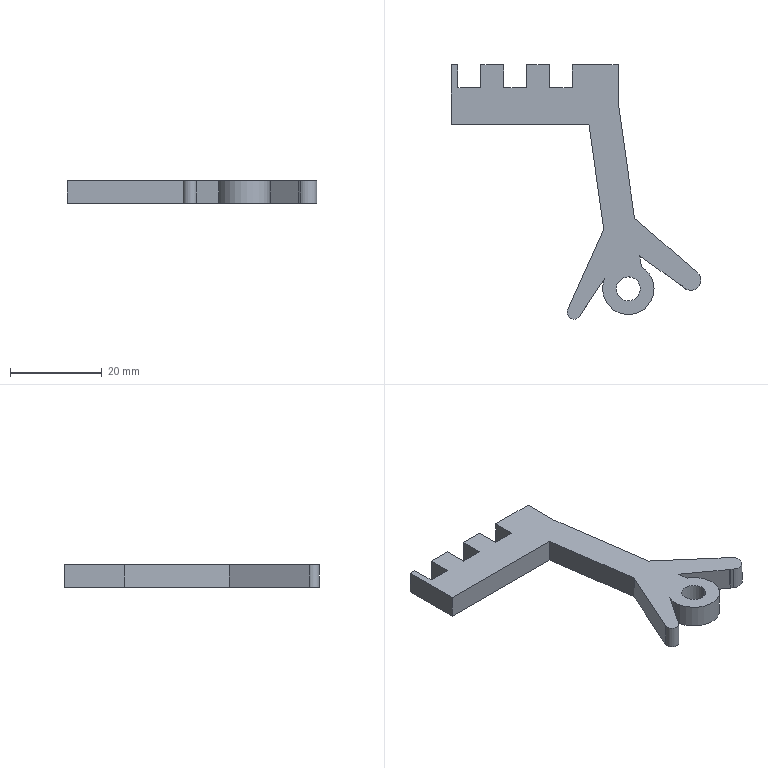Part | SolidWorks | features ICE 28, Join 2 | 1 solid | 34 faces | box 54.608 x 55.606 x 5 mm | volume 4241 mm3 | plane 27 | cylinder 7 | commonest cylinder face diameters 11.246 x3 5.25 x2 3 x1 4.42 x1
STEP:
#1=CARTESIAN_POINT('',(28.531,-18.492,-5.));
#2=VERTEX_POINT('',#1);
#3=CARTESIAN_POINT('',(28.044,-20.781,-5.));
#4=VERTEX_POINT('',#3);
#5=CARTESIAN_POINT('',(33.667,-20.781,-5.));
#6=DIRECTION('',(0.,0.,1.));
#7=DIRECTION('',(-1.,0.,0.));
#8=AXIS2_PLACEMENT_3D('',#5,#6,#7);
#9=CIRCLE('',#8,5.623);
#10=EDGE_CURVE('',#2,#4,#9,.T.);
#11=ORIENTED_EDGE('',*,*,#10,.T.);
#12=CARTESIAN_POINT('',(28.044,-20.781,0.));
#13=VERTEX_POINT('',#12);
#14=CARTESIAN_POINT('',(28.044,-20.781,-20.904));
#15=DIRECTION('',(0.,0.,1.));
#16=VECTOR('',#15,1000.);
#17=LINE('',#14,#16);
#18=EDGE_CURVE('',#4,#13,#17,.T.);
#19=ORIENTED_EDGE('',*,*,#18,.T.);
#20=CARTESIAN_POINT('',(28.531,-18.492,0.));
#21=VERTEX_POINT('',#20);
#22=CARTESIAN_POINT('',(33.667,-20.781,0.));
#23=DIRECTION('',(0.,0.,1.));
#24=DIRECTION('',(1.,0.,0.));
#25=AXIS2_PLACEMENT_3D('',#22,#23,#24);
#26=CIRCLE('',#25,5.623);
#27=EDGE_CURVE('',#21,#13,#26,.T.);
#28=ORIENTED_EDGE('',*,*,#27,.F.);
#29=CARTESIAN_POINT('',(28.531,-18.492,-20.904));
#30=DIRECTION('',(0.,0.,-1.));
#31=VECTOR('',#30,1000.);
#32=LINE('',#29,#31);
#33=EDGE_CURVE('',#21,#2,#32,.T.);
#34=ORIENTED_EDGE('',*,*,#33,.T.);
#35=EDGE_LOOP('',(#11,#19,#28,#34));
#36=FACE_OUTER_BOUND('',#35,.T.);
#37=CARTESIAN_POINT('',(33.667,-20.781,-20.904));
#38=DIRECTION('',(0.,0.,1.));
#39=DIRECTION('',(1.,0.,0.));
#40=AXIS2_PLACEMENT_3D('',#37,#38,#39);
#41=CYLINDRICAL_SURFACE('',#40,5.623);
#42=ADVANCED_FACE('',(#36),#41,.T.);
#43=ORIENTED_EDGE('',*,*,#18,.F.);
#44=CARTESIAN_POINT('',(39.29,-20.781,-5.));
#45=VERTEX_POINT('',#44);
#46=CARTESIAN_POINT('',(33.667,-20.781,-5.));
#47=DIRECTION('',(0.,0.,1.));
#48=DIRECTION('',(-1.,0.,0.));
#49=AXIS2_PLACEMENT_3D('',#46,#47,#48);
#50=CIRCLE('',#49,5.623);
#51=EDGE_CURVE('',#4,#45,#50,.T.);
#52=ORIENTED_EDGE('',*,*,#51,.T.);
#53=CARTESIAN_POINT('',(39.29,-20.781,0.));
#54=VERTEX_POINT('',#53);
#55=CARTESIAN_POINT('',(39.29,-20.781,-20.904));
#56=DIRECTION('',(0.,0.,1.));
#57=VECTOR('',#56,1000.);
#58=LINE('',#55,#57);
#59=EDGE_CURVE('',#45,#54,#58,.T.);
#60=ORIENTED_EDGE('',*,*,#59,.T.);
#61=CARTESIAN_POINT('',(33.667,-20.781,0.));
#62=DIRECTION('',(0.,0.,1.));
#63=DIRECTION('',(1.,0.,0.));
#64=AXIS2_PLACEMENT_3D('',#61,#62,#63);
#65=CIRCLE('',#64,5.623);
#66=EDGE_CURVE('',#13,#54,#65,.T.);
#67=ORIENTED_EDGE('',*,*,#66,.F.);
#68=EDGE_LOOP('',(#43,#52,#60,#67));
#69=FACE_OUTER_BOUND('',#68,.T.);
#70=CARTESIAN_POINT('',(33.667,-20.781,-20.904));
#71=DIRECTION('',(0.,0.,1.));
#72=DIRECTION('',(1.,0.,0.));
#73=AXIS2_PLACEMENT_3D('',#70,#71,#72);
#74=CYLINDRICAL_SURFACE('',#73,5.623);
#75=ADVANCED_FACE('',(#69),#74,.T.);
#76=CARTESIAN_POINT('',(36.277,-21.054,-5.));
#77=VERTEX_POINT('',#76);
#78=CARTESIAN_POINT('',(31.056,-20.508,-5.));
#79=VERTEX_POINT('',#78);
#80=CARTESIAN_POINT('',(33.667,-20.781,-5.));
#81=DIRECTION('',(0.,0.,-1.));
#82=DIRECTION('',(-0.9946,0.1041,0.));
#83=AXIS2_PLACEMENT_3D('',#80,#81,#82);
#84=CIRCLE('',#83,2.625);
#85=EDGE_CURVE('',#77,#79,#84,.T.);
#86=ORIENTED_EDGE('',*,*,#85,.T.);
#87=CARTESIAN_POINT('',(31.056,-20.508,0.));
#88=VERTEX_POINT('',#87);
#89=CARTESIAN_POINT('',(31.056,-20.508,-10.));
#90=DIRECTION('',(0.,0.,1.));
#91=VECTOR('',#90,1000.);
#92=LINE('',#89,#91);
#93=EDGE_CURVE('',#79,#88,#92,.T.);
#94=ORIENTED_EDGE('',*,*,#93,.T.);
#95=CARTESIAN_POINT('',(36.277,-21.054,0.));
#96=VERTEX_POINT('',#95);
#97=CARTESIAN_POINT('',(33.667,-20.781,0.));
#98=DIRECTION('',(0.,0.,1.));
#99=DIRECTION('',(0.9946,-0.1041,0.));
#100=AXIS2_PLACEMENT_3D('',#97,#98,#99);
#101=CIRCLE('',#100,2.625);
#102=EDGE_CURVE('',#88,#96,#101,.T.);
#103=ORIENTED_EDGE('',*,*,#102,.T.);
#104=CARTESIAN_POINT('',(36.277,-21.054,-10.));
#105=DIRECTION('',(0.,0.,1.));
#106=VECTOR('',#105,1000.);
#107=LINE('',#104,#106);
#108=EDGE_CURVE('',#77,#96,#107,.T.);
#109=ORIENTED_EDGE('',*,*,#108,.F.);
#110=EDGE_LOOP('',(#86,#94,#103,#109));
#111=FACE_OUTER_BOUND('',#110,.T.);
#112=CARTESIAN_POINT('',(33.667,-20.781,-10.));
#113=DIRECTION('',(0.,0.,1.));
#114=DIRECTION('',(0.9946,-0.1041,0.));
#115=AXIS2_PLACEMENT_3D('',#112,#113,#114);
#116=CYLINDRICAL_SURFACE('',#115,2.625);
#117=ADVANCED_FACE('',(#111),#116,.F.);
#118=CARTESIAN_POINT('',(-5.057,28.192,0.));
#119=VERTEX_POINT('',#118);
#120=CARTESIAN_POINT('',(-5.057,28.192,-5.));
#121=VERTEX_POINT('',#120);
#122=CARTESIAN_POINT('',(-5.057,28.192,5.));
#123=DIRECTION('',(0.,0.,-1.));
#124=VECTOR('',#123,1000.);
#125=LINE('',#122,#124);
#126=EDGE_CURVE('',#119,#121,#125,.T.);
#127=ORIENTED_EDGE('',*,*,#126,.F.);
#128=CARTESIAN_POINT('',(-3.557,28.192,0.));
#129=VERTEX_POINT('',#128);
#130=CARTESIAN_POINT('',(-16.089,28.192,0.));
#131=DIRECTION('',(1.,0.,0.));
#132=VECTOR('',#131,1000.);
#133=LINE('',#130,#132);
#134=EDGE_CURVE('',#119,#129,#133,.T.);
#135=ORIENTED_EDGE('',*,*,#134,.T.);
#136=CARTESIAN_POINT('',(-3.557,28.192,-5.));
#137=VERTEX_POINT('',#136);
#138=CARTESIAN_POINT('',(-3.557,28.192,0.001));
#139=DIRECTION('',(0.,0.,-1.));
#140=VECTOR('',#139,1000.);
#141=LINE('',#138,#140);
#142=EDGE_CURVE('',#129,#137,#141,.T.);
#143=ORIENTED_EDGE('',*,*,#142,.T.);
#144=CARTESIAN_POINT('',(-16.089,28.192,-5.));
#145=DIRECTION('',(1.,0.,0.));
#146=VECTOR('',#145,1000.);
#147=LINE('',#144,#146);
#148=EDGE_CURVE('',#121,#137,#147,.T.);
#149=ORIENTED_EDGE('',*,*,#148,.F.);
#150=EDGE_LOOP('',(#127,#135,#143,#149));
#151=FACE_OUTER_BOUND('',#150,.T.);
#152=CARTESIAN_POINT('',(-16.089,28.192,-5.));
#153=DIRECTION('',(0.,-1.,0.));
#154=DIRECTION('',(0.,0.,-1.));
#155=AXIS2_PLACEMENT_3D('',#152,#153,#154);
#156=PLANE('',#155);
#157=ADVANCED_FACE('',(#151),#156,.F.);
#158=CARTESIAN_POINT('',(-5.057,15.192,0.));
#159=VERTEX_POINT('',#158);
#160=CARTESIAN_POINT('',(-5.057,15.192,-5.));
#161=VERTEX_POINT('',#160);
#162=CARTESIAN_POINT('',(-5.057,15.192,5.));
#163=DIRECTION('',(0.,0.,-1.));
#164=VECTOR('',#163,1000.);
#165=LINE('',#162,#164);
#166=EDGE_CURVE('',#159,#161,#165,.T.);
#167=ORIENTED_EDGE('',*,*,#166,.T.);
#168=CARTESIAN_POINT('',(25.077,15.192,-5.));
#169=VERTEX_POINT('',#168);
#170=CARTESIAN_POINT('',(-16.089,15.192,-5.));
#171=DIRECTION('',(1.,0.,0.));
#172=VECTOR('',#171,1000.);
#173=LINE('',#170,#172);
#174=EDGE_CURVE('',#161,#169,#173,.T.);
#175=ORIENTED_EDGE('',*,*,#174,.T.);
#176=CARTESIAN_POINT('',(25.077,15.192,0.));
#177=VERTEX_POINT('',#176);
#178=CARTESIAN_POINT('',(25.077,15.192,0.));
#179=DIRECTION('',(0.,0.,-1.));
#180=VECTOR('',#179,1000.);
#181=LINE('',#178,#180);
#182=EDGE_CURVE('',#177,#169,#181,.T.);
#183=ORIENTED_EDGE('',*,*,#182,.F.);
#184=CARTESIAN_POINT('',(-16.089,15.192,0.));
#185=DIRECTION('',(1.,0.,0.));
#186=VECTOR('',#185,1000.);
#187=LINE('',#184,#186);
#188=EDGE_CURVE('',#159,#177,#187,.T.);
#189=ORIENTED_EDGE('',*,*,#188,.F.);
#190=EDGE_LOOP('',(#167,#175,#183,#189));
#191=FACE_OUTER_BOUND('',#190,.T.);
#192=CARTESIAN_POINT('',(-16.089,15.192,-5.));
#193=DIRECTION('',(0.,1.,0.));
#194=DIRECTION('',(0.,0.,1.));
#195=AXIS2_PLACEMENT_3D('',#192,#193,#194);
#196=PLANE('',#195);
#197=ADVANCED_FACE('',(#191),#196,.F.);
#198=CARTESIAN_POINT('',(46.044,-20.68,-5.));
#199=VERTEX_POINT('',#198);
#200=CARTESIAN_POINT('',(48.785,-17.218,-5.));
#201=VERTEX_POINT('',#200);
#202=CARTESIAN_POINT('',(47.341,-18.89,-5.));
#203=DIRECTION('',(0.,0.,1.));
#204=DIRECTION('',(-1.,0.,0.));
#205=AXIS2_PLACEMENT_3D('',#202,#203,#204);
#206=CIRCLE('',#205,2.21);
#207=EDGE_CURVE('',#199,#201,#206,.T.);
#208=ORIENTED_EDGE('',*,*,#207,.F.);
#209=CARTESIAN_POINT('',(45.413,-20.127,-5.));
#210=VERTEX_POINT('',#209);
#211=CARTESIAN_POINT('',(45.413,-20.127,-5.));
#212=DIRECTION('',(0.7522,-0.6589,0.));
#213=VECTOR('',#212,1000.);
#214=LINE('',#211,#213);
#215=EDGE_CURVE('',#210,#199,#214,.T.);
#216=ORIENTED_EDGE('',*,*,#215,.F.);
#217=CARTESIAN_POINT('',(45.451,-20.251,-5.));
#218=VERTEX_POINT('',#217);
#219=CARTESIAN_POINT('',(46.236,-22.795,-5.));
#220=DIRECTION('',(-0.2947,0.9556,0.));
#221=VECTOR('',#220,1000.);
#222=LINE('',#219,#221);
#223=EDGE_CURVE('',#218,#210,#222,.T.);
#224=ORIENTED_EDGE('',*,*,#223,.F.);
#225=CARTESIAN_POINT('',(36.183,-13.539,-5.));
#226=VERTEX_POINT('',#225);
#227=CARTESIAN_POINT('',(3.892,9.847,-5.));
#228=DIRECTION('',(-0.8099,0.5865,0.));
#229=VECTOR('',#228,1000.);
#230=LINE('',#227,#229);
#231=EDGE_CURVE('',#218,#226,#230,.T.);
#232=ORIENTED_EDGE('',*,*,#231,.T.);
#233=CARTESIAN_POINT('',(36.52,-15.936,-5.));
#234=VERTEX_POINT('',#233);
#235=CARTESIAN_POINT('',(37.552,-23.275,-5.));
#236=DIRECTION('',(-0.1392,0.9903,0.));
#237=VECTOR('',#236,1000.);
#238=LINE('',#235,#237);
#239=EDGE_CURVE('',#234,#226,#238,.T.);
#240=ORIENTED_EDGE('',*,*,#239,.F.);
#241=CARTESIAN_POINT('',(33.667,-20.781,-5.));
#242=DIRECTION('',(0.,0.,1.));
#243=DIRECTION('',(-1.,0.,0.));
#244=AXIS2_PLACEMENT_3D('',#241,#242,#243);
#245=CIRCLE('',#244,5.623);
#246=EDGE_CURVE('',#45,#234,#245,.T.);
#247=ORIENTED_EDGE('',*,*,#246,.F.);
#248=ORIENTED_EDGE('',*,*,#51,.F.);
#249=ORIENTED_EDGE('',*,*,#10,.F.);
#250=CARTESIAN_POINT('',(23.157,-26.529,-5.));
#251=VERTEX_POINT('',#250);
#252=CARTESIAN_POINT('',(23.157,-26.529,-5.));
#253=DIRECTION('',(0.5558,0.8313,0.));
#254=VECTOR('',#253,1000.);
#255=LINE('',#252,#254);
#256=EDGE_CURVE('',#251,#2,#255,.T.);
#257=ORIENTED_EDGE('',*,*,#256,.F.);
#258=CARTESIAN_POINT('',(20.421,-25.3,-5.));
#259=VERTEX_POINT('',#258);
#260=CARTESIAN_POINT('',(21.789,-25.914,-5.));
#261=DIRECTION('',(0.,0.,1.));
#262=DIRECTION('',(0.9903,0.1392,0.));
#263=AXIS2_PLACEMENT_3D('',#260,#261,#262);
#264=CIRCLE('',#263,1.5);
#265=EDGE_CURVE('',#259,#251,#264,.T.);
#266=ORIENTED_EDGE('',*,*,#265,.F.);
#267=CARTESIAN_POINT('',(28.302,-7.759,-5.));
#268=VERTEX_POINT('',#267);
#269=CARTESIAN_POINT('',(28.302,-7.759,-5.));
#270=DIRECTION('',(-0.4099,-0.9121,0.));
#271=VECTOR('',#270,1000.);
#272=LINE('',#269,#271);
#273=EDGE_CURVE('',#268,#259,#272,.T.);
#274=ORIENTED_EDGE('',*,*,#273,.F.);
#275=CARTESIAN_POINT('',(30.62,-24.249,-5.));
#276=DIRECTION('',(0.1392,-0.9903,0.));
#277=VECTOR('',#276,1000.);
#278=LINE('',#275,#277);
#279=EDGE_CURVE('',#169,#268,#278,.T.);
#280=ORIENTED_EDGE('',*,*,#279,.F.);
#281=ORIENTED_EDGE('',*,*,#174,.F.);
#282=CARTESIAN_POINT('',(-5.057,0.,-5.));
#283=DIRECTION('',(0.,1.,0.));
#284=VECTOR('',#283,1000.);
#285=LINE('',#282,#284);
#286=EDGE_CURVE('',#161,#121,#285,.T.);
#287=ORIENTED_EDGE('',*,*,#286,.T.);
#288=ORIENTED_EDGE('',*,*,#148,.T.);
#289=CARTESIAN_POINT('',(-3.557,23.192,-5.));
#290=VERTEX_POINT('',#289);
#291=CARTESIAN_POINT('',(-3.557,28.192,-5.));
#292=DIRECTION('',(0.,1.,0.));
#293=VECTOR('',#292,1000.);
#294=LINE('',#291,#293);
#295=EDGE_CURVE('',#290,#137,#294,.T.);
#296=ORIENTED_EDGE('',*,*,#295,.F.);
#297=CARTESIAN_POINT('',(1.443,23.192,-5.));
#298=VERTEX_POINT('',#297);
#299=CARTESIAN_POINT('',(1.443,23.192,-5.));
#300=DIRECTION('',(-1.,0.,0.));
#301=VECTOR('',#300,1000.);
#302=LINE('',#299,#301);
#303=EDGE_CURVE('',#298,#290,#302,.T.);
#304=ORIENTED_EDGE('',*,*,#303,.F.);
#305=CARTESIAN_POINT('',(1.443,28.192,-5.));
#306=VERTEX_POINT('',#305);
#307=CARTESIAN_POINT('',(1.443,28.192,-5.));
#308=DIRECTION('',(0.,-1.,0.));
#309=VECTOR('',#308,1000.);
#310=LINE('',#307,#309);
#311=EDGE_CURVE('',#306,#298,#310,.T.);
#312=ORIENTED_EDGE('',*,*,#311,.F.);
#313=CARTESIAN_POINT('',(6.443,28.192,-5.));
#314=VERTEX_POINT('',#313);
#315=CARTESIAN_POINT('',(-16.089,28.192,-5.));
#316=DIRECTION('',(1.,0.,0.));
#317=VECTOR('',#316,1000.);
#318=LINE('',#315,#317);
#319=EDGE_CURVE('',#306,#314,#318,.T.);
#320=ORIENTED_EDGE('',*,*,#319,.T.);
#321=CARTESIAN_POINT('',(6.443,23.192,-5.));
#322=VERTEX_POINT('',#321);
#323=CARTESIAN_POINT('',(6.443,28.192,-5.));
#324=DIRECTION('',(0.,1.,0.));
#325=VECTOR('',#324,1000.);
#326=LINE('',#323,#325);
#327=EDGE_CURVE('',#322,#314,#326,.T.);
#328=ORIENTED_EDGE('',*,*,#327,.F.);
#329=CARTESIAN_POINT('',(11.443,23.192,-5.));
#330=VERTEX_POINT('',#329);
#331=CARTESIAN_POINT('',(6.443,23.192,-5.));
#332=DIRECTION('',(-1.,0.,0.));
#333=VECTOR('',#332,1000.);
#334=LINE('',#331,#333);
#335=EDGE_CURVE('',#330,#322,#334,.T.);
#336=ORIENTED_EDGE('',*,*,#335,.F.);
#337=CARTESIAN_POINT('',(11.443,28.192,-5.));
#338=VERTEX_POINT('',#337);
#339=CARTESIAN_POINT('',(11.443,28.192,-5.));
#340=DIRECTION('',(0.,-1.,0.));
#341=VECTOR('',#340,1000.);
#342=LINE('',#339,#341);
#343=EDGE_CURVE('',#338,#330,#342,.T.);
#344=ORIENTED_EDGE('',*,*,#343,.F.);
#345=CARTESIAN_POINT('',(16.443,28.192,-5.));
#346=VERTEX_POINT('',#345);
#347=CARTESIAN_POINT('',(-16.089,28.192,-5.));
#348=DIRECTION('',(1.,0.,0.));
#349=VECTOR('',#348,1000.);
#350=LINE('',#347,#349);
#351=EDGE_CURVE('',#338,#346,#350,.T.);
#352=ORIENTED_EDGE('',*,*,#351,.T.);
#353=CARTESIAN_POINT('',(16.443,23.192,-5.));
#354=VERTEX_POINT('',#353);
#355=CARTESIAN_POINT('',(16.443,28.192,-5.));
#356=DIRECTION('',(0.,1.,0.));
#357=VECTOR('',#356,1000.);
#358=LINE('',#355,#357);
#359=EDGE_CURVE('',#354,#346,#358,.T.);
#360=ORIENTED_EDGE('',*,*,#359,.F.);
#361=CARTESIAN_POINT('',(21.443,23.192,-5.));
#362=VERTEX_POINT('',#361);
#363=CARTESIAN_POINT('',(16.443,23.192,-5.));
#364=DIRECTION('',(-1.,0.,0.));
#365=VECTOR('',#364,1000.);
#366=LINE('',#363,#365);
#367=EDGE_CURVE('',#362,#354,#366,.T.);
#368=ORIENTED_EDGE('',*,*,#367,.F.);
#369=CARTESIAN_POINT('',(21.443,28.192,-5.));
#370=VERTEX_POINT('',#369);
#371=CARTESIAN_POINT('',(21.443,28.192,-5.));
#372=DIRECTION('',(0.,-1.,0.));
#373=VECTOR('',#372,1000.);
#374=LINE('',#371,#373);
#375=EDGE_CURVE('',#370,#362,#374,.T.);
#376=ORIENTED_EDGE('',*,*,#375,.F.);
#377=CARTESIAN_POINT('',(31.443,28.192,-5.));
#378=VERTEX_POINT('',#377);
#379=CARTESIAN_POINT('',(-16.089,28.192,-5.));
#380=DIRECTION('',(1.,0.,0.));
#381=VECTOR('',#380,1000.);
#382=LINE('',#379,#381);
#383=EDGE_CURVE('',#370,#378,#382,.T.);
#384=ORIENTED_EDGE('',*,*,#383,.T.);
#385=CARTESIAN_POINT('',(31.443,20.192,-5.));
#386=VERTEX_POINT('',#385);
#387=CARTESIAN_POINT('',(31.443,28.192,-5.));
#388=DIRECTION('',(0.,1.,0.));
#389=VECTOR('',#388,1000.);
#390=LINE('',#387,#389);
#391=EDGE_CURVE('',#386,#378,#390,.T.);
#392=ORIENTED_EDGE('',*,*,#391,.F.);
#393=CARTESIAN_POINT('',(35.031,-5.339,-5.));
#394=VERTEX_POINT('',#393);
#395=CARTESIAN_POINT('',(32.145,15.192,-5.));
#396=DIRECTION('',(-0.1392,0.9903,0.));
#397=VECTOR('',#396,1000.);
#398=LINE('',#395,#397);
#399=EDGE_CURVE('',#394,#386,#398,.T.);
#400=ORIENTED_EDGE('',*,*,#399,.F.);
#401=CARTESIAN_POINT('',(10.255,16.058,-5.));
#402=DIRECTION('',(0.7568,-0.6536,0.));
#403=VECTOR('',#402,1000.);
#404=LINE('',#401,#403);
#405=EDGE_CURVE('',#394,#201,#404,.T.);
#406=ORIENTED_EDGE('',*,*,#405,.T.);
#407=EDGE_LOOP('',(#208,#216,#224,#232,#240,#247,#248,#249,#257,#266,#274,#280,#281,#287,#288,#296,#304,#312,#320,#328,#336,#344,#352,#360,#368,#376,#384,#392,#400,#406));
#408=FACE_OUTER_BOUND('',#407,.T.);
#409=ORIENTED_EDGE('',*,*,#85,.F.);
#410=CARTESIAN_POINT('',(33.667,-20.781,-5.));
#411=DIRECTION('',(0.,0.,-1.));
#412=DIRECTION('',(-0.9946,0.1041,0.));
#413=AXIS2_PLACEMENT_3D('',#410,#411,#412);
#414=CIRCLE('',#413,2.625);
#415=EDGE_CURVE('',#79,#77,#414,.T.);
#416=ORIENTED_EDGE('',*,*,#415,.F.);
#417=EDGE_LOOP('',(#409,#416));
#418=FACE_BOUND('',#417,.T.);
#419=CARTESIAN_POINT('',(33.02,-2.82,-5.));
#420=DIRECTION('',(0.,0.,-1.));
#421=DIRECTION('',(-0.9704,-0.2415,0.));
#422=AXIS2_PLACEMENT_3D('',#419,#420,#421);
#423=PLANE('',#422);
#424=ADVANCED_FACE('',(#408,#418),#423,.T.);
#425=CARTESIAN_POINT('',(33.667,-20.781,0.));
#426=DIRECTION('',(0.,0.,1.));
#427=DIRECTION('',(0.9946,-0.1041,0.));
#428=AXIS2_PLACEMENT_3D('',#425,#426,#427);
#429=CIRCLE('',#428,2.625);
#430=EDGE_CURVE('',#96,#88,#429,.T.);
#431=ORIENTED_EDGE('',*,*,#430,.F.);
#432=ORIENTED_EDGE('',*,*,#102,.F.);
#433=EDGE_LOOP('',(#431,#432));
#434=FACE_BOUND('',#433,.T.);
#435=CARTESIAN_POINT('',(45.413,-20.127,0.));
#436=VERTEX_POINT('',#435);
#437=CARTESIAN_POINT('',(46.044,-20.68,0.));
#438=VERTEX_POINT('',#437);
#439=CARTESIAN_POINT('',(45.413,-20.127,0.));
#440=DIRECTION('',(0.7522,-0.6589,0.));
#441=VECTOR('',#440,1000.);
#442=LINE('',#439,#441);
#443=EDGE_CURVE('',#436,#438,#442,.T.);
#444=ORIENTED_EDGE('',*,*,#443,.T.);
#445=CARTESIAN_POINT('',(48.785,-17.218,0.));
#446=VERTEX_POINT('',#445);
#447=CARTESIAN_POINT('',(47.341,-18.89,0.));
#448=DIRECTION('',(0.,0.,1.));
#449=DIRECTION('',(-1.,0.,0.));
#450=AXIS2_PLACEMENT_3D('',#447,#448,#449);
#451=CIRCLE('',#450,2.21);
#452=EDGE_CURVE('',#438,#446,#451,.T.);
#453=ORIENTED_EDGE('',*,*,#452,.T.);
#454=CARTESIAN_POINT('',(35.031,-5.339,0.));
#455=VERTEX_POINT('',#454);
#456=CARTESIAN_POINT('',(10.255,16.058,0.));
#457=DIRECTION('',(0.7568,-0.6536,0.));
#458=VECTOR('',#457,1000.);
#459=LINE('',#456,#458);
#460=EDGE_CURVE('',#455,#446,#459,.T.);
#461=ORIENTED_EDGE('',*,*,#460,.F.);
#462=CARTESIAN_POINT('',(31.443,20.192,0.));
#463=VERTEX_POINT('',#462);
#464=CARTESIAN_POINT('',(32.145,15.192,0.));
#465=DIRECTION('',(-0.1392,0.9903,0.));
#466=VECTOR('',#465,1000.);
#467=LINE('',#464,#466);
#468=EDGE_CURVE('',#455,#463,#467,.T.);
#469=ORIENTED_EDGE('',*,*,#468,.T.);
#470=CARTESIAN_POINT('',(31.443,28.192,0.));
#471=VERTEX_POINT('',#470);
#472=CARTESIAN_POINT('',(31.443,28.192,0.));
#473=DIRECTION('',(0.,1.,0.));
#474=VECTOR('',#473,1000.);
#475=LINE('',#472,#474);
#476=EDGE_CURVE('',#463,#471,#475,.T.);
#477=ORIENTED_EDGE('',*,*,#476,.T.);
#478=CARTESIAN_POINT('',(21.443,28.192,0.));
#479=VERTEX_POINT('',#478);
#480=CARTESIAN_POINT('',(-16.089,28.192,0.));
#481=DIRECTION('',(1.,0.,0.));
#482=VECTOR('',#481,1000.);
#483=LINE('',#480,#482);
#484=EDGE_CURVE('',#479,#471,#483,.T.);
#485=ORIENTED_EDGE('',*,*,#484,.F.);
#486=CARTESIAN_POINT('',(21.443,23.192,0.));
#487=VERTEX_POINT('',#486);
#488=CARTESIAN_POINT('',(21.443,28.192,0.));
#489=DIRECTION('',(0.,1.,0.));
#490=VECTOR('',#489,1000.);
#491=LINE('',#488,#490);
#492=EDGE_CURVE('',#487,#479,#491,.T.);
#493=ORIENTED_EDGE('',*,*,#492,.F.);
#494=CARTESIAN_POINT('',(16.443,23.192,0.));
#495=VERTEX_POINT('',#494);
#496=CARTESIAN_POINT('',(16.443,23.192,0.));
#497=DIRECTION('',(1.,0.,0.));
#498=VECTOR('',#497,1000.);
#499=LINE('',#496,#498);
#500=EDGE_CURVE('',#495,#487,#499,.T.);
#501=ORIENTED_EDGE('',*,*,#500,.F.);
#502=CARTESIAN_POINT('',(16.443,28.192,0.));
#503=VERTEX_POINT('',#502);
#504=CARTESIAN_POINT('',(16.443,28.192,0.));
#505=DIRECTION('',(0.,-1.,0.));
#506=VECTOR('',#505,1000.);
#507=LINE('',#504,#506);
#508=EDGE_CURVE('',#503,#495,#507,.T.);
#509=ORIENTED_EDGE('',*,*,#508,.F.);
#510=CARTESIAN_POINT('',(11.443,28.192,0.));
#511=VERTEX_POINT('',#510);
#512=CARTESIAN_POINT('',(-16.089,28.192,0.));
#513=DIRECTION('',(1.,0.,0.));
#514=VECTOR('',#513,1000.);
#515=LINE('',#512,#514);
#516=EDGE_CURVE('',#511,#503,#515,.T.);
#517=ORIENTED_EDGE('',*,*,#516,.F.);
#518=CARTESIAN_POINT('',(11.443,23.192,0.));
#519=VERTEX_POINT('',#518);
#520=CARTESIAN_POINT('',(11.443,28.192,0.));
#521=DIRECTION('',(0.,1.,0.));
#522=VECTOR('',#521,1000.);
#523=LINE('',#520,#522);
#524=EDGE_CURVE('',#519,#511,#523,.T.);
#525=ORIENTED_EDGE('',*,*,#524,.F.);
#526=CARTESIAN_POINT('',(6.443,23.192,0.));
#527=VERTEX_POINT('',#526);
#528=CARTESIAN_POINT('',(6.443,23.192,0.));
#529=DIRECTION('',(1.,0.,0.));
#530=VECTOR('',#529,1000.);
#531=LINE('',#528,#530);
#532=EDGE_CURVE('',#527,#519,#531,.T.);
#533=ORIENTED_EDGE('',*,*,#532,.F.);
#534=CARTESIAN_POINT('',(6.443,28.192,0.));
#535=VERTEX_POINT('',#534);
#536=CARTESIAN_POINT('',(6.443,28.192,0.));
#537=DIRECTION('',(0.,-1.,0.));
#538=VECTOR('',#537,1000.);
#539=LINE('',#536,#538);
#540=EDGE_CURVE('',#535,#527,#539,.T.);
#541=ORIENTED_EDGE('',*,*,#540,.F.);
#542=CARTESIAN_POINT('',(1.443,28.192,0.));
#543=VERTEX_POINT('',#542);
#544=CARTESIAN_POINT('',(-16.089,28.192,0.));
#545=DIRECTION('',(1.,0.,0.));
#546=VECTOR('',#545,1000.);
#547=LINE('',#544,#546);
#548=EDGE_CURVE('',#543,#535,#547,.T.);
#549=ORIENTED_EDGE('',*,*,#548,.F.);
#550=CARTESIAN_POINT('',(1.443,23.192,0.));
#551=VERTEX_POINT('',#550);
#552=CARTESIAN_POINT('',(1.443,28.192,0.));
#553=DIRECTION('',(0.,1.,0.));
#554=VECTOR('',#553,1000.);
#555=LINE('',#552,#554);
#556=EDGE_CURVE('',#551,#543,#555,.T.);
#557=ORIENTED_EDGE('',*,*,#556,.F.);
#558=CARTESIAN_POINT('',(-3.557,23.192,0.));
#559=VERTEX_POINT('',#558);
#560=CARTESIAN_POINT('',(1.443,23.192,0.));
#561=DIRECTION('',(1.,0.,0.));
#562=VECTOR('',#561,1000.);
#563=LINE('',#560,#562);
#564=EDGE_CURVE('',#559,#551,#563,.T.);
#565=ORIENTED_EDGE('',*,*,#564,.F.);
#566=CARTESIAN_POINT('',(-3.557,28.192,0.));
#567=DIRECTION('',(0.,-1.,0.));
#568=VECTOR('',#567,1000.);
#569=LINE('',#566,#568);
#570=EDGE_CURVE('',#129,#559,#569,.T.);
#571=ORIENTED_EDGE('',*,*,#570,.F.);
#572=ORIENTED_EDGE('',*,*,#134,.F.);
#573=CARTESIAN_POINT('',(-5.057,-2.82,0.));
#574=DIRECTION('',(0.,1.,0.));
#575=VECTOR('',#574,1000.);
#576=LINE('',#573,#575);
#577=EDGE_CURVE('',#159,#119,#576,.T.);
#578=ORIENTED_EDGE('',*,*,#577,.F.);
#579=ORIENTED_EDGE('',*,*,#188,.T.);
#580=CARTESIAN_POINT('',(28.302,-7.759,0.));
#581=VERTEX_POINT('',#580);
#582=CARTESIAN_POINT('',(30.62,-24.249,0.));
#583=DIRECTION('',(0.1392,-0.9903,0.));
#584=VECTOR('',#583,1000.);
#585=LINE('',#582,#584);
#586=EDGE_CURVE('',#177,#581,#585,.T.);
#587=ORIENTED_EDGE('',*,*,#586,.T.);
#588=CARTESIAN_POINT('',(20.421,-25.3,0.));
#589=VERTEX_POINT('',#588);
#590=CARTESIAN_POINT('',(28.302,-7.759,0.));
#591=DIRECTION('',(-0.4099,-0.9121,0.));
#592=VECTOR('',#591,1000.);
#593=LINE('',#590,#592);
#594=EDGE_CURVE('',#581,#589,#593,.T.);
#595=ORIENTED_EDGE('',*,*,#594,.T.);
#596=CARTESIAN_POINT('',(23.157,-26.529,0.));
#597=VERTEX_POINT('',#596);
#598=CARTESIAN_POINT('',(21.789,-25.914,0.));
#599=DIRECTION('',(0.,0.,1.));
#600=DIRECTION('',(0.9903,0.1392,0.));
#601=AXIS2_PLACEMENT_3D('',#598,#599,#600);
#602=CIRCLE('',#601,1.5);
#603=EDGE_CURVE('',#589,#597,#602,.T.);
#604=ORIENTED_EDGE('',*,*,#603,.T.);
#605=CARTESIAN_POINT('',(23.157,-26.529,0.));
#606=DIRECTION('',(0.5558,0.8313,0.));
#607=VECTOR('',#606,1000.);
#608=LINE('',#605,#607);
#609=EDGE_CURVE('',#597,#21,#608,.T.);
#610=ORIENTED_EDGE('',*,*,#609,.T.);
#611=ORIENTED_EDGE('',*,*,#27,.T.);
#612=ORIENTED_EDGE('',*,*,#66,.T.);
#613=CARTESIAN_POINT('',(36.52,-15.936,0.));
#614=VERTEX_POINT('',#613);
#615=CARTESIAN_POINT('',(33.667,-20.781,0.));
#616=DIRECTION('',(0.,0.,1.));
#617=DIRECTION('',(1.,0.,0.));
#618=AXIS2_PLACEMENT_3D('',#615,#616,#617);
#619=CIRCLE('',#618,5.623);
#620=EDGE_CURVE('',#54,#614,#619,.T.);
#621=ORIENTED_EDGE('',*,*,#620,.T.);
#622=CARTESIAN_POINT('',(36.183,-13.539,0.));
#623=VERTEX_POINT('',#622);
#624=CARTESIAN_POINT('',(37.552,-23.275,0.));
#625=DIRECTION('',(-0.1392,0.9903,0.));
#626=VECTOR('',#625,1000.);
#627=LINE('',#624,#626);
#628=EDGE_CURVE('',#614,#623,#627,.T.);
#629=ORIENTED_EDGE('',*,*,#628,.T.);
#630=CARTESIAN_POINT('',(45.451,-20.251,0.));
#631=VERTEX_POINT('',#630);
#632=CARTESIAN_POINT('',(3.892,9.847,0.));
#633=DIRECTION('',(-0.8099,0.5865,0.));
#634=VECTOR('',#633,1000.);
#635=LINE('',#632,#634);
#636=EDGE_CURVE('',#631,#623,#635,.T.);
#637=ORIENTED_EDGE('',*,*,#636,.F.);
#638=CARTESIAN_POINT('',(46.236,-22.795,0.));
#639=DIRECTION('',(-0.2947,0.9556,0.));
#640=VECTOR('',#639,1000.);
#641=LINE('',#638,#640);
#642=EDGE_CURVE('',#631,#436,#641,.T.);
#643=ORIENTED_EDGE('',*,*,#642,.T.);
#644=EDGE_LOOP('',(#444,#453,#461,#469,#477,#485,#493,#501,#509,#517,#525,#533,#541,#549,#557,#565,#571,#572,#578,#579,#587,#595,#604,#610,#611,#612,#621,#629,#637,#643));
#645=FACE_OUTER_BOUND('',#644,.T.);
#646=CARTESIAN_POINT('',(33.02,-2.82,0.));
#647=DIRECTION('',(0.,0.,-1.));
#648=DIRECTION('',(-0.9704,-0.2415,0.));
#649=AXIS2_PLACEMENT_3D('',#646,#647,#648);
#650=PLANE('',#649);
#651=ADVANCED_FACE('',(#434,#645),#650,.F.);
#652=ORIENTED_EDGE('',*,*,#516,.T.);
#653=CARTESIAN_POINT('',(16.443,28.192,0.001));
#654=DIRECTION('',(0.,0.,-1.));
#655=VECTOR('',#654,1000.);
#656=LINE('',#653,#655);
#657=EDGE_CURVE('',#503,#346,#656,.T.);
#658=ORIENTED_EDGE('',*,*,#657,.T.);
#659=ORIENTED_EDGE('',*,*,#351,.F.);
#660=CARTESIAN_POINT('',(11.443,28.192,0.001));
#661=DIRECTION('',(0.,0.,-1.));
#662=VECTOR('',#661,1000.);
#663=LINE('',#660,#662);
#664=EDGE_CURVE('',#511,#338,#663,.T.);
#665=ORIENTED_EDGE('',*,*,#664,.F.);
#666=EDGE_LOOP('',(#652,#658,#659,#665));
#667=FACE_OUTER_BOUND('',#666,.T.);
#668=CARTESIAN_POINT('',(-16.089,28.192,-5.));
#669=DIRECTION('',(0.,-1.,0.));
#670=DIRECTION('',(0.,0.,-1.));
#671=AXIS2_PLACEMENT_3D('',#668,#669,#670);
#672=PLANE('',#671);
#673=ADVANCED_FACE('',(#667),#672,.F.);
#674=ORIENTED_EDGE('',*,*,#319,.F.);
#675=CARTESIAN_POINT('',(1.443,28.192,0.001));
#676=DIRECTION('',(0.,0.,-1.));
#677=VECTOR('',#676,1000.);
#678=LINE('',#675,#677);
#679=EDGE_CURVE('',#543,#306,#678,.T.);
#680=ORIENTED_EDGE('',*,*,#679,.F.);
#681=ORIENTED_EDGE('',*,*,#548,.T.);
#682=CARTESIAN_POINT('',(6.443,28.192,0.001));
#683=DIRECTION('',(0.,0.,-1.));
#684=VECTOR('',#683,1000.);
#685=LINE('',#682,#684);
#686=EDGE_CURVE('',#535,#314,#685,.T.);
#687=ORIENTED_EDGE('',*,*,#686,.T.);
#688=EDGE_LOOP('',(#674,#680,#681,#687));
#689=FACE_OUTER_BOUND('',#688,.T.);
#690=CARTESIAN_POINT('',(-16.089,28.192,-5.));
#691=DIRECTION('',(0.,-1.,0.));
#692=DIRECTION('',(0.,0.,-1.));
#693=AXIS2_PLACEMENT_3D('',#690,#691,#692);
#694=PLANE('',#693);
#695=ADVANCED_FACE('',(#689),#694,.F.);
#696=ORIENTED_EDGE('',*,*,#383,.F.);
#697=CARTESIAN_POINT('',(21.443,28.192,0.001));
#698=DIRECTION('',(0.,0.,-1.));
#699=VECTOR('',#698,1000.);
#700=LINE('',#697,#699);
#701=EDGE_CURVE('',#479,#370,#700,.T.);
#702=ORIENTED_EDGE('',*,*,#701,.F.);
#703=ORIENTED_EDGE('',*,*,#484,.T.);
#704=CARTESIAN_POINT('',(31.443,28.192,-13.391));
#705=DIRECTION('',(0.,0.,1.));
#706=VECTOR('',#705,1000.);
#707=LINE('',#704,#706);
#708=EDGE_CURVE('',#378,#471,#707,.T.);
#709=ORIENTED_EDGE('',*,*,#708,.F.);
#710=EDGE_LOOP('',(#696,#702,#703,#709));
#711=FACE_OUTER_BOUND('',#710,.T.);
#712=CARTESIAN_POINT('',(-16.089,28.192,-5.));
#713=DIRECTION('',(0.,-1.,0.));
#714=DIRECTION('',(0.,0.,-1.));
#715=AXIS2_PLACEMENT_3D('',#712,#713,#714);
#716=PLANE('',#715);
#717=ADVANCED_FACE('',(#711),#716,.F.);
#718=ORIENTED_EDGE('',*,*,#468,.F.);
#719=CARTESIAN_POINT('',(35.031,-5.339,-5.));
#720=DIRECTION('',(0.,0.,1.));
#721=VECTOR('',#720,1000.);
#722=LINE('',#719,#721);
#723=EDGE_CURVE('',#394,#455,#722,.T.);
#724=ORIENTED_EDGE('',*,*,#723,.F.);
#725=ORIENTED_EDGE('',*,*,#399,.T.);
#726=CARTESIAN_POINT('',(31.443,20.192,-5.));
#727=DIRECTION('',(0.,0.,1.));
#728=VECTOR('',#727,1000.);
#729=LINE('',#726,#728);
#730=EDGE_CURVE('',#386,#463,#729,.T.);
#731=ORIENTED_EDGE('',*,*,#730,.T.);
#732=EDGE_LOOP('',(#718,#724,#725,#731));
#733=FACE_OUTER_BOUND('',#732,.T.);
#734=CARTESIAN_POINT('',(32.145,15.192,-5.));
#735=DIRECTION('',(0.9903,0.1392,0.));
#736=DIRECTION('',(-0.1392,0.9903,0.));
#737=AXIS2_PLACEMENT_3D('',#734,#735,#736);
#738=PLANE('',#737);
#739=ADVANCED_FACE('',(#733),#738,.T.);
#740=ORIENTED_EDGE('',*,*,#628,.F.);
#741=CARTESIAN_POINT('',(36.52,-15.936,-20.904));
#742=DIRECTION('',(0.,0.,-1.));
#743=VECTOR('',#742,1000.);
#744=LINE('',#741,#743);
#745=EDGE_CURVE('',#614,#234,#744,.T.);
#746=ORIENTED_EDGE('',*,*,#745,.T.);
#747=ORIENTED_EDGE('',*,*,#239,.T.);
#748=CARTESIAN_POINT('',(36.183,-13.539,-5.));
#749=DIRECTION('',(0.,0.,1.));
#750=VECTOR('',#749,1000.);
#751=LINE('',#748,#750);
#752=EDGE_CURVE('',#226,#623,#751,.T.);
#753=ORIENTED_EDGE('',*,*,#752,.T.);
#754=EDGE_LOOP('',(#740,#746,#747,#753));
#755=FACE_OUTER_BOUND('',#754,.T.);
#756=CARTESIAN_POINT('',(37.552,-23.275,0.));
#757=DIRECTION('',(-0.9903,-0.1392,0.));
#758=DIRECTION('',(0.,0.,1.));
#759=AXIS2_PLACEMENT_3D('',#756,#757,#758);
#760=PLANE('',#759);
#761=ADVANCED_FACE('',(#755),#760,.F.);
#762=ORIENTED_EDGE('',*,*,#594,.F.);
#763=CARTESIAN_POINT('',(28.302,-7.759,-5.));
#764=DIRECTION('',(0.,0.,1.));
#765=VECTOR('',#764,1000.);
#766=LINE('',#763,#765);
#767=EDGE_CURVE('',#268,#581,#766,.T.);
#768=ORIENTED_EDGE('',*,*,#767,.F.);
#769=ORIENTED_EDGE('',*,*,#273,.T.);
#770=CARTESIAN_POINT('',(20.421,-25.3,-5.));
#771=DIRECTION('',(0.,0.,1.));
#772=VECTOR('',#771,1000.);
#773=LINE('',#770,#772);
#774=EDGE_CURVE('',#259,#589,#773,.T.);
#775=ORIENTED_EDGE('',*,*,#774,.T.);
#776=EDGE_LOOP('',(#762,#768,#769,#775));
#777=FACE_OUTER_BOUND('',#776,.T.);
#778=CARTESIAN_POINT('',(28.302,-7.759,-5.));
#779=DIRECTION('',(-0.9121,0.4099,0.));
#780=DIRECTION('',(-0.4099,-0.9121,0.));
#781=AXIS2_PLACEMENT_3D('',#778,#779,#780);
#782=PLANE('',#781);
#783=ADVANCED_FACE('',(#777),#782,.T.);
#784=ORIENTED_EDGE('',*,*,#603,.F.);
#785=ORIENTED_EDGE('',*,*,#774,.F.);
#786=ORIENTED_EDGE('',*,*,#265,.T.);
#787=CARTESIAN_POINT('',(23.157,-26.529,-5.));
#788=DIRECTION('',(0.,0.,1.));
#789=VECTOR('',#788,1000.);
#790=LINE('',#787,#789);
#791=EDGE_CURVE('',#251,#597,#790,.T.);
#792=ORIENTED_EDGE('',*,*,#791,.T.);
#793=EDGE_LOOP('',(#784,#785,#786,#792));
#794=FACE_OUTER_BOUND('',#793,.T.);
#795=CARTESIAN_POINT('',(21.789,-25.914,-5.));
#796=DIRECTION('',(0.,0.,1.));
#797=DIRECTION('',(0.9903,0.1392,0.));
#798=AXIS2_PLACEMENT_3D('',#795,#796,#797);
#799=CYLINDRICAL_SURFACE('',#798,1.5);
#800=ADVANCED_FACE('',(#794),#799,.T.);
#801=ORIENTED_EDGE('',*,*,#33,.F.);
#802=ORIENTED_EDGE('',*,*,#609,.F.);
#803=ORIENTED_EDGE('',*,*,#791,.F.);
#804=ORIENTED_EDGE('',*,*,#256,.T.);
#805=EDGE_LOOP('',(#801,#802,#803,#804));
#806=FACE_OUTER_BOUND('',#805,.T.);
#807=CARTESIAN_POINT('',(23.157,-26.529,-5.));
#808=DIRECTION('',(0.8313,-0.5558,0.));
#809=DIRECTION('',(0.5558,0.8313,0.));
#810=AXIS2_PLACEMENT_3D('',#807,#808,#809);
#811=PLANE('',#810);
#812=ADVANCED_FACE('',(#806),#811,.T.);
#813=ORIENTED_EDGE('',*,*,#586,.F.);
#814=ORIENTED_EDGE('',*,*,#182,.T.);
#815=ORIENTED_EDGE('',*,*,#279,.T.);
#816=ORIENTED_EDGE('',*,*,#767,.T.);
#817=EDGE_LOOP('',(#813,#814,#815,#816));
#818=FACE_OUTER_BOUND('',#817,.T.);
#819=CARTESIAN_POINT('',(30.62,-24.249,0.));
#820=DIRECTION('',(0.9903,0.1392,0.));
#821=DIRECTION('',(0.,0.,-1.));
#822=AXIS2_PLACEMENT_3D('',#819,#820,#821);
#823=PLANE('',#822);
#824=ADVANCED_FACE('',(#818),#823,.F.);
#825=ORIENTED_EDGE('',*,*,#231,.F.);
#826=CARTESIAN_POINT('',(45.451,-20.251,-5.));
#827=DIRECTION('',(0.,0.,1.));
#828=VECTOR('',#827,1000.);
#829=LINE('',#826,#828);
#830=EDGE_CURVE('',#218,#631,#829,.T.);
#831=ORIENTED_EDGE('',*,*,#830,.T.);
#832=ORIENTED_EDGE('',*,*,#636,.T.);
#833=ORIENTED_EDGE('',*,*,#752,.F.);
#834=EDGE_LOOP('',(#825,#831,#832,#833));
#835=FACE_OUTER_BOUND('',#834,.T.);
#836=CARTESIAN_POINT('',(3.892,9.847,-5.));
#837=DIRECTION('',(0.5865,0.8099,0.));
#838=DIRECTION('',(-0.8099,0.5865,0.));
#839=AXIS2_PLACEMENT_3D('',#836,#837,#838);
#840=PLANE('',#839);
#841=ADVANCED_FACE('',(#835),#840,.F.);
#842=ORIENTED_EDGE('',*,*,#460,.T.);
#843=CARTESIAN_POINT('',(48.785,-17.218,0.));
#844=DIRECTION('',(0.,0.,-1.));
#845=VECTOR('',#844,1000.);
#846=LINE('',#843,#845);
#847=EDGE_CURVE('',#446,#201,#846,.T.);
#848=ORIENTED_EDGE('',*,*,#847,.T.);
#849=ORIENTED_EDGE('',*,*,#405,.F.);
#850=ORIENTED_EDGE('',*,*,#723,.T.);
#851=EDGE_LOOP('',(#842,#848,#849,#850));
#852=FACE_OUTER_BOUND('',#851,.T.);
#853=CARTESIAN_POINT('',(10.255,16.058,-5.));
#854=DIRECTION('',(-0.6536,-0.7568,0.));
#855=DIRECTION('',(0.7568,-0.6536,0.));
#856=AXIS2_PLACEMENT_3D('',#853,#854,#855);
#857=PLANE('',#856);
#858=ADVANCED_FACE('',(#852),#857,.F.);
#859=ORIENTED_EDGE('',*,*,#93,.F.);
#860=ORIENTED_EDGE('',*,*,#415,.T.);
#861=ORIENTED_EDGE('',*,*,#108,.T.);
#862=ORIENTED_EDGE('',*,*,#430,.T.);
#863=EDGE_LOOP('',(#859,#860,#861,#862));
#864=FACE_OUTER_BOUND('',#863,.T.);
#865=CARTESIAN_POINT('',(33.667,-20.781,-10.));
#866=DIRECTION('',(0.,0.,1.));
#867=DIRECTION('',(0.9946,-0.1041,0.));
#868=AXIS2_PLACEMENT_3D('',#865,#866,#867);
#869=CYLINDRICAL_SURFACE('',#868,2.625);
#870=ADVANCED_FACE('',(#864),#869,.F.);
#871=ORIENTED_EDGE('',*,*,#59,.F.);
#872=ORIENTED_EDGE('',*,*,#246,.T.);
#873=ORIENTED_EDGE('',*,*,#745,.F.);
#874=ORIENTED_EDGE('',*,*,#620,.F.);
#875=EDGE_LOOP('',(#871,#872,#873,#874));
#876=FACE_OUTER_BOUND('',#875,.T.);
#877=CARTESIAN_POINT('',(33.667,-20.781,-20.904));
#878=DIRECTION('',(0.,0.,1.));
#879=DIRECTION('',(1.,0.,0.));
#880=AXIS2_PLACEMENT_3D('',#877,#878,#879);
#881=CYLINDRICAL_SURFACE('',#880,5.623);
#882=ADVANCED_FACE('',(#876),#881,.T.);
#883=ORIENTED_EDGE('',*,*,#730,.F.);
#884=ORIENTED_EDGE('',*,*,#391,.T.);
#885=ORIENTED_EDGE('',*,*,#708,.T.);
#886=ORIENTED_EDGE('',*,*,#476,.F.);
#887=EDGE_LOOP('',(#883,#884,#885,#886));
#888=FACE_OUTER_BOUND('',#887,.T.);
#889=CARTESIAN_POINT('',(31.443,28.192,-13.391));
#890=DIRECTION('',(1.,0.,0.));
#891=DIRECTION('',(0.,0.,-1.));
#892=AXIS2_PLACEMENT_3D('',#889,#890,#891);
#893=PLANE('',#892);
#894=ADVANCED_FACE('',(#888),#893,.T.);
#895=ORIENTED_EDGE('',*,*,#540,.T.);
#896=CARTESIAN_POINT('',(6.443,23.192,0.001));
#897=DIRECTION('',(0.,0.,-1.));
#898=VECTOR('',#897,1000.);
#899=LINE('',#896,#898);
#900=EDGE_CURVE('',#527,#322,#899,.T.);
#901=ORIENTED_EDGE('',*,*,#900,.T.);
#902=ORIENTED_EDGE('',*,*,#327,.T.);
#903=ORIENTED_EDGE('',*,*,#686,.F.);
#904=EDGE_LOOP('',(#895,#901,#902,#903));
#905=FACE_OUTER_BOUND('',#904,.T.);
#906=CARTESIAN_POINT('',(6.443,28.192,0.001));
#907=DIRECTION('',(-1.,0.,0.));
#908=DIRECTION('',(0.,-1.,0.));
#909=AXIS2_PLACEMENT_3D('',#906,#907,#908);
#910=PLANE('',#909);
#911=ADVANCED_FACE('',(#905),#910,.F.);
#912=ORIENTED_EDGE('',*,*,#532,.T.);
#913=CARTESIAN_POINT('',(11.443,23.192,0.001));
#914=DIRECTION('',(0.,0.,-1.));
#915=VECTOR('',#914,1000.);
#916=LINE('',#913,#915);
#917=EDGE_CURVE('',#519,#330,#916,.T.);
#918=ORIENTED_EDGE('',*,*,#917,.T.);
#919=ORIENTED_EDGE('',*,*,#335,.T.);
#920=ORIENTED_EDGE('',*,*,#900,.F.);
#921=EDGE_LOOP('',(#912,#918,#919,#920));
#922=FACE_OUTER_BOUND('',#921,.T.);
#923=CARTESIAN_POINT('',(6.443,23.192,0.001));
#924=DIRECTION('',(0.,-1.,0.));
#925=DIRECTION('',(1.,0.,0.));
#926=AXIS2_PLACEMENT_3D('',#923,#924,#925);
#927=PLANE('',#926);
#928=ADVANCED_FACE('',(#922),#927,.F.);
#929=ORIENTED_EDGE('',*,*,#524,.T.);
#930=ORIENTED_EDGE('',*,*,#664,.T.);
#931=ORIENTED_EDGE('',*,*,#343,.T.);
#932=ORIENTED_EDGE('',*,*,#917,.F.);
#933=EDGE_LOOP('',(#929,#930,#931,#932));
#934=FACE_OUTER_BOUND('',#933,.T.);
#935=CARTESIAN_POINT('',(11.443,28.192,0.001));
#936=DIRECTION('',(1.,0.,0.));
#937=DIRECTION('',(0.,0.,-1.));
#938=AXIS2_PLACEMENT_3D('',#935,#936,#937);
#939=PLANE('',#938);
#940=ADVANCED_FACE('',(#934),#939,.F.);
#941=ORIENTED_EDGE('',*,*,#556,.T.);
#942=ORIENTED_EDGE('',*,*,#679,.T.);
#943=ORIENTED_EDGE('',*,*,#311,.T.);
#944=CARTESIAN_POINT('',(1.443,23.192,0.001));
#945=DIRECTION('',(0.,0.,-1.));
#946=VECTOR('',#945,1000.);
#947=LINE('',#944,#946);
#948=EDGE_CURVE('',#551,#298,#947,.T.);
#949=ORIENTED_EDGE('',*,*,#948,.F.);
#950=EDGE_LOOP('',(#941,#942,#943,#949));
#951=FACE_OUTER_BOUND('',#950,.T.);
#952=CARTESIAN_POINT('',(1.443,28.192,0.001));
#953=DIRECTION('',(1.,0.,0.));
#954=DIRECTION('',(0.,1.,0.));
#955=AXIS2_PLACEMENT_3D('',#952,#953,#954);
#956=PLANE('',#955);
#957=ADVANCED_FACE('',(#951),#956,.F.);
#958=ORIENTED_EDGE('',*,*,#570,.T.);
#959=CARTESIAN_POINT('',(-3.557,23.192,0.001));
#960=DIRECTION('',(0.,0.,-1.));
#961=VECTOR('',#960,1000.);
#962=LINE('',#959,#961);
#963=EDGE_CURVE('',#559,#290,#962,.T.);
#964=ORIENTED_EDGE('',*,*,#963,.T.);
#965=ORIENTED_EDGE('',*,*,#295,.T.);
#966=ORIENTED_EDGE('',*,*,#142,.F.);
#967=EDGE_LOOP('',(#958,#964,#965,#966));
#968=FACE_OUTER_BOUND('',#967,.T.);
#969=CARTESIAN_POINT('',(-3.557,28.192,0.001));
#970=DIRECTION('',(-1.,0.,0.));
#971=DIRECTION('',(0.,0.,1.));
#972=AXIS2_PLACEMENT_3D('',#969,#970,#971);
#973=PLANE('',#972);
#974=ADVANCED_FACE('',(#968),#973,.F.);
#975=ORIENTED_EDGE('',*,*,#564,.T.);
#976=ORIENTED_EDGE('',*,*,#948,.T.);
#977=ORIENTED_EDGE('',*,*,#303,.T.);
#978=ORIENTED_EDGE('',*,*,#963,.F.);
#979=EDGE_LOOP('',(#975,#976,#977,#978));
#980=FACE_OUTER_BOUND('',#979,.T.);
#981=CARTESIAN_POINT('',(1.443,23.192,0.001));
#982=DIRECTION('',(0.,-1.,0.));
#983=DIRECTION('',(0.,0.,-1.));
#984=AXIS2_PLACEMENT_3D('',#981,#982,#983);
#985=PLANE('',#984);
#986=ADVANCED_FACE('',(#980),#985,.F.);
#987=ORIENTED_EDGE('',*,*,#508,.T.);
#988=CARTESIAN_POINT('',(16.443,23.192,0.001));
#989=DIRECTION('',(0.,0.,-1.));
#990=VECTOR('',#989,1000.);
#991=LINE('',#988,#990);
#992=EDGE_CURVE('',#495,#354,#991,.T.);
#993=ORIENTED_EDGE('',*,*,#992,.T.);
#994=ORIENTED_EDGE('',*,*,#359,.T.);
#995=ORIENTED_EDGE('',*,*,#657,.F.);
#996=EDGE_LOOP('',(#987,#993,#994,#995));
#997=FACE_OUTER_BOUND('',#996,.T.);
#998=CARTESIAN_POINT('',(16.443,28.192,0.001));
#999=DIRECTION('',(-1.,0.,0.));
#1000=DIRECTION('',(0.,0.,1.));
#1001=AXIS2_PLACEMENT_3D('',#998,#999,#1000);
#1002=PLANE('',#1001);
#1003=ADVANCED_FACE('',(#997),#1002,.F.);
#1004=ORIENTED_EDGE('',*,*,#500,.T.);
#1005=CARTESIAN_POINT('',(21.443,23.192,0.001));
#1006=DIRECTION('',(0.,0.,-1.));
#1007=VECTOR('',#1006,1000.);
#1008=LINE('',#1005,#1007);
#1009=EDGE_CURVE('',#487,#362,#1008,.T.);
#1010=ORIENTED_EDGE('',*,*,#1009,.T.);
#1011=ORIENTED_EDGE('',*,*,#367,.T.);
#1012=ORIENTED_EDGE('',*,*,#992,.F.);
#1013=EDGE_LOOP('',(#1004,#1010,#1011,#1012));
#1014=FACE_OUTER_BOUND('',#1013,.T.);
#1015=CARTESIAN_POINT('',(16.443,23.192,0.001));
#1016=DIRECTION('',(0.,-1.,0.));
#1017=DIRECTION('',(0.,0.,-1.));
#1018=AXIS2_PLACEMENT_3D('',#1015,#1016,#1017);
#1019=PLANE('',#1018);
#1020=ADVANCED_FACE('',(#1014),#1019,.F.);
#1021=ORIENTED_EDGE('',*,*,#492,.T.);
#1022=ORIENTED_EDGE('',*,*,#701,.T.);
#1023=ORIENTED_EDGE('',*,*,#375,.T.);
#1024=ORIENTED_EDGE('',*,*,#1009,.F.);
#1025=EDGE_LOOP('',(#1021,#1022,#1023,#1024));
#1026=FACE_OUTER_BOUND('',#1025,.T.);
#1027=CARTESIAN_POINT('',(21.443,28.192,0.001));
#1028=DIRECTION('',(1.,0.,0.));
#1029=DIRECTION('',(0.,0.,-1.));
#1030=AXIS2_PLACEMENT_3D('',#1027,#1028,#1029);
#1031=PLANE('',#1030);
#1032=ADVANCED_FACE('',(#1026),#1031,.F.);
#1033=ORIENTED_EDGE('',*,*,#577,.T.);
#1034=ORIENTED_EDGE('',*,*,#126,.T.);
#1035=ORIENTED_EDGE('',*,*,#286,.F.);
#1036=ORIENTED_EDGE('',*,*,#166,.F.);
#1037=EDGE_LOOP('',(#1033,#1034,#1035,#1036));
#1038=FACE_OUTER_BOUND('',#1037,.T.);
#1039=CARTESIAN_POINT('',(-5.057,0.,5.));
#1040=DIRECTION('',(-1.,0.,0.));
#1041=DIRECTION('',(0.,0.,1.));
#1042=AXIS2_PLACEMENT_3D('',#1039,#1040,#1041);
#1043=PLANE('',#1042);
#1044=ADVANCED_FACE('',(#1038),#1043,.T.);
#1045=ORIENTED_EDGE('',*,*,#223,.T.);
#1046=CARTESIAN_POINT('',(45.413,-20.127,0.));
#1047=DIRECTION('',(0.,0.,-1.));
#1048=VECTOR('',#1047,1000.);
#1049=LINE('',#1046,#1048);
#1050=EDGE_CURVE('',#436,#210,#1049,.T.);
#1051=ORIENTED_EDGE('',*,*,#1050,.F.);
#1052=ORIENTED_EDGE('',*,*,#642,.F.);
#1053=ORIENTED_EDGE('',*,*,#830,.F.);
#1054=EDGE_LOOP('',(#1045,#1051,#1052,#1053));
#1055=FACE_OUTER_BOUND('',#1054,.T.);
#1056=CARTESIAN_POINT('',(46.236,-22.795,0.));
#1057=DIRECTION('',(-0.9556,-0.2947,0.));
#1058=DIRECTION('',(0.2947,-0.9556,0.));
#1059=AXIS2_PLACEMENT_3D('',#1056,#1057,#1058);
#1060=PLANE('',#1059);
#1061=ADVANCED_FACE('',(#1055),#1060,.F.);
#1062=ORIENTED_EDGE('',*,*,#207,.T.);
#1063=ORIENTED_EDGE('',*,*,#847,.F.);
#1064=ORIENTED_EDGE('',*,*,#452,.F.);
#1065=CARTESIAN_POINT('',(46.044,-20.68,0.));
#1066=DIRECTION('',(0.,0.,-1.));
#1067=VECTOR('',#1066,1000.);
#1068=LINE('',#1065,#1067);
#1069=EDGE_CURVE('',#438,#199,#1068,.T.);
#1070=ORIENTED_EDGE('',*,*,#1069,.T.);
#1071=EDGE_LOOP('',(#1062,#1063,#1064,#1070));
#1072=FACE_OUTER_BOUND('',#1071,.T.);
#1073=CARTESIAN_POINT('',(47.341,-18.89,0.));
#1074=DIRECTION('',(0.,0.,-1.));
#1075=DIRECTION('',(-1.,0.,0.));
#1076=AXIS2_PLACEMENT_3D('',#1073,#1074,#1075);
#1077=CYLINDRICAL_SURFACE('',#1076,2.21);
#1078=ADVANCED_FACE('',(#1072),#1077,.T.);
#1079=ORIENTED_EDGE('',*,*,#215,.T.);
#1080=ORIENTED_EDGE('',*,*,#1069,.F.);
#1081=ORIENTED_EDGE('',*,*,#443,.F.);
#1082=ORIENTED_EDGE('',*,*,#1050,.T.);
#1083=EDGE_LOOP('',(#1079,#1080,#1081,#1082));
#1084=FACE_OUTER_BOUND('',#1083,.T.);
#1085=CARTESIAN_POINT('',(45.413,-20.127,0.));
#1086=DIRECTION('',(0.6589,0.7522,0.));
#1087=DIRECTION('',(-0.7522,0.6589,0.));
#1088=AXIS2_PLACEMENT_3D('',#1085,#1086,#1087);
#1089=PLANE('',#1088);
#1090=ADVANCED_FACE('',(#1084),#1089,.F.);
#1091=CLOSED_SHELL('',(#42,#75,#117,#157,#197,#424,#651,#673,#695,#717,#739,#761,#783,#800,#812,#824,#841,#858,#870,#882,#894,#911,#928,#940,#957,#974,#986,#1003,#1020,#1032,#1044,#1061,#1078,#1090));
#1092=MANIFOLD_SOLID_BREP('',#1091);
#1093=CARTESIAN_POINT('',(0.,0.,0.));
#1094=DIRECTION('',(0.,0.,1.));
#1095=DIRECTION('',(1.,0.,0.));
#1096=AXIS2_PLACEMENT_3D('',#1093,#1094,#1095);
#1097=(LENGTH_UNIT()NAMED_UNIT(*)SI_UNIT(.MILLI.,.METRE.));
#1098=UNCERTAINTY_MEASURE_WITH_UNIT(LENGTH_MEASURE(0.00001),#1097,'','');
#1099=(NAMED_UNIT(*)PLANE_ANGLE_UNIT()SI_UNIT($,.RADIAN.));
#1100=(NAMED_UNIT(*)SI_UNIT($,.STERADIAN.)SOLID_ANGLE_UNIT());
#1101=(GEOMETRIC_REPRESENTATION_CONTEXT(3)GLOBAL_UNCERTAINTY_ASSIGNED_CONTEXT((#1098))GLOBAL_UNIT_ASSIGNED_CONTEXT((#1097,#1099,#1100))REPRESENTATION_CONTEXT('',''));
#1102=ADVANCED_BREP_SHAPE_REPRESENTATION('',(#1092,#1096),#1101);